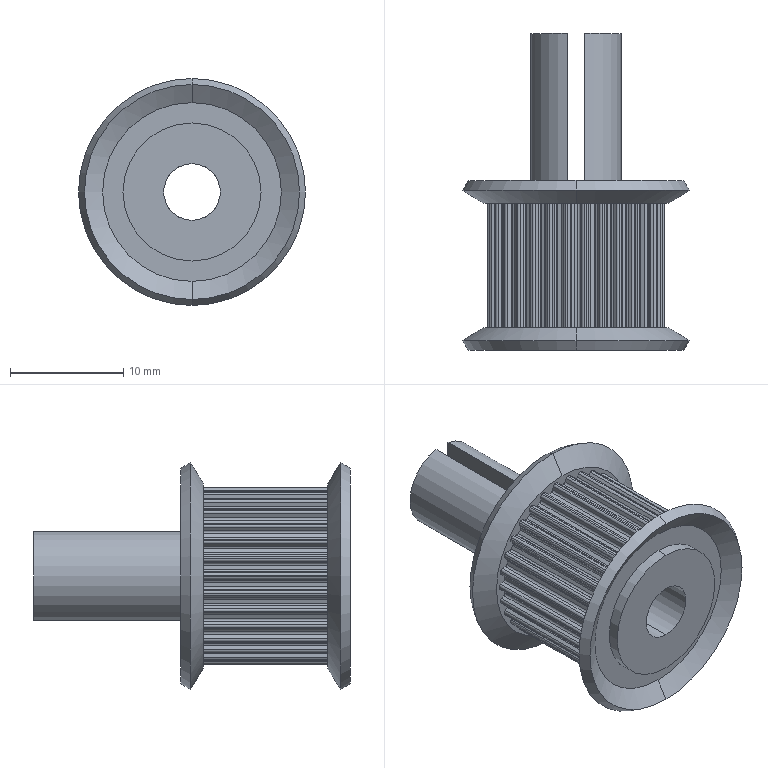Part | NX | features BREP 1 | 1 solid | 294 faces | box 20.061 x 28 x 20.061 mm | volume 2842 mm3 | cylinder 180 | plane 102 | cone 12 | commonest cylinder face diameters 0.46 x142 15.66 x30 12.2 x4 5 x2 8 x2